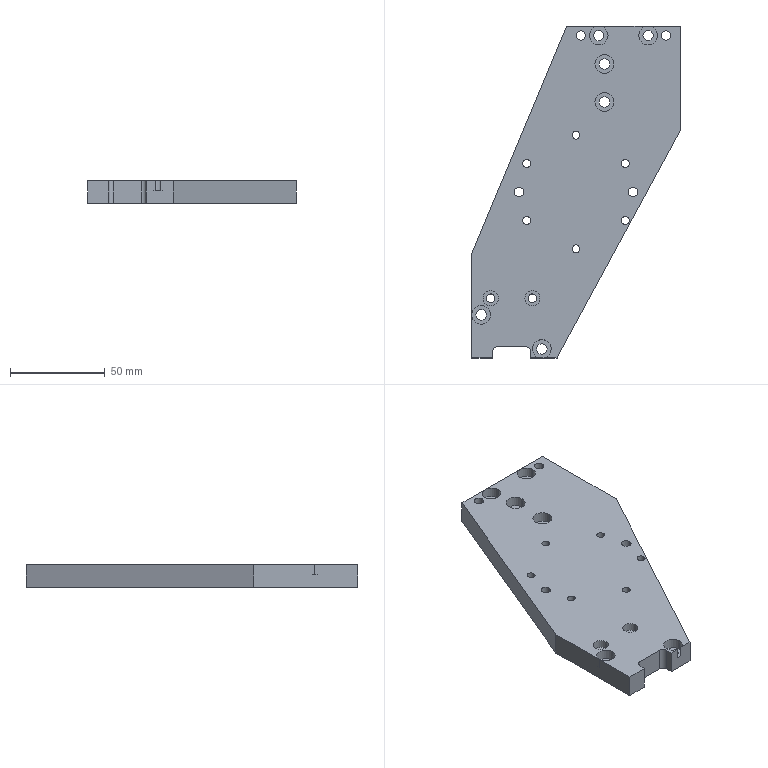Part | SolidWorks | features HoleWzd 7, Chamfer 2, Extrusion 1, Fillet 1, ICE 1, RefAxis 1 | 1 solid | 75 faces | box 110 x 175 x 12 mm | volume 140751 mm3 | cylinder 55 | plane 20 | commonest cylinder face diameters 4.2 x12 5.5 x12 5 x10 9.8 x9 4.5 x4 8 x4